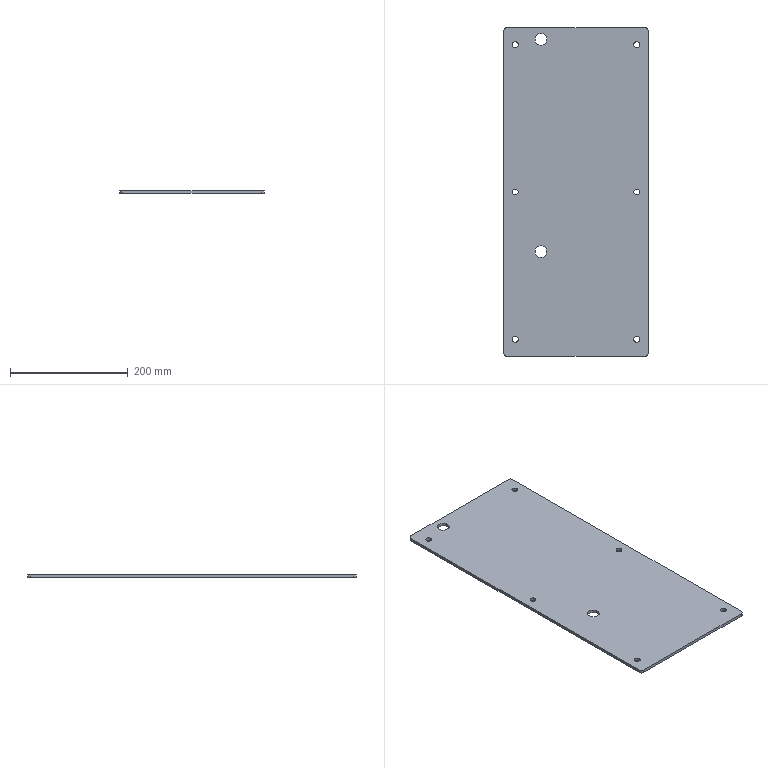Part | SolidWorks | features BaseBody 1 | 1 solid | 26 faces | box 244.5 x 558 x 5 mm | volume 676550 mm3 | cylinder 20 | plane 6 | commonest cylinder face diameters 10 x16 20 x4
STEP:
#1=CARTESIAN_POINT('',(-49.502,-101.,5.));
#2=VERTEX_POINT('',#1);
#3=CARTESIAN_POINT('',(-69.502,-101.,5.));
#4=VERTEX_POINT('',#3);
#5=CARTESIAN_POINT('',(-59.502,-101.,5.));
#6=DIRECTION('',(0.,0.,-1.));
#7=DIRECTION('',(-1.,0.,0.));
#8=AXIS2_PLACEMENT_3D('',#5,#6,#7);
#9=CIRCLE('',#8,10.);
#10=EDGE_CURVE('',#2,#4,#9,.T.);
#11=ORIENTED_EDGE('',*,*,#10,.F.);
#12=CARTESIAN_POINT('',(-49.502,-101.,0.));
#13=VERTEX_POINT('',#12);
#14=CARTESIAN_POINT('',(-49.502,-101.,10.));
#15=DIRECTION('',(0.,0.,-1.));
#16=VECTOR('',#15,1000.);
#17=LINE('',#14,#16);
#18=EDGE_CURVE('',#2,#13,#17,.T.);
#19=ORIENTED_EDGE('',*,*,#18,.T.);
#20=CARTESIAN_POINT('',(-69.502,-101.,0.));
#21=VERTEX_POINT('',#20);
#22=CARTESIAN_POINT('',(-59.502,-101.,0.));
#23=DIRECTION('',(0.,0.,-1.));
#24=DIRECTION('',(-1.,0.,0.));
#25=AXIS2_PLACEMENT_3D('',#22,#23,#24);
#26=CIRCLE('',#25,10.);
#27=EDGE_CURVE('',#13,#21,#26,.T.);
#28=ORIENTED_EDGE('',*,*,#27,.T.);
#29=CARTESIAN_POINT('',(-69.502,-101.,10.));
#30=DIRECTION('',(0.,0.,-1.));
#31=VECTOR('',#30,1000.);
#32=LINE('',#29,#31);
#33=EDGE_CURVE('',#4,#21,#32,.T.);
#34=ORIENTED_EDGE('',*,*,#33,.F.);
#35=EDGE_LOOP('',(#11,#19,#28,#34));
#36=FACE_OUTER_BOUND('',#35,.T.);
#37=CARTESIAN_POINT('',(-59.502,-101.,10.));
#38=DIRECTION('',(0.,0.,-1.));
#39=DIRECTION('',(-1.,0.,0.));
#40=AXIS2_PLACEMENT_3D('',#37,#38,#39);
#41=CYLINDRICAL_SURFACE('',#40,10.);
#42=ADVANCED_FACE('',(#36),#41,.F.);
#43=CARTESIAN_POINT('',(-49.502,259.,5.));
#44=VERTEX_POINT('',#43);
#45=CARTESIAN_POINT('',(-69.502,259.,5.));
#46=VERTEX_POINT('',#45);
#47=CARTESIAN_POINT('',(-59.502,259.,5.));
#48=DIRECTION('',(0.,0.,-1.));
#49=DIRECTION('',(-1.,0.,0.));
#50=AXIS2_PLACEMENT_3D('',#47,#48,#49);
#51=CIRCLE('',#50,10.);
#52=EDGE_CURVE('',#44,#46,#51,.T.);
#53=ORIENTED_EDGE('',*,*,#52,.F.);
#54=CARTESIAN_POINT('',(-49.502,259.,0.));
#55=VERTEX_POINT('',#54);
#56=CARTESIAN_POINT('',(-49.502,259.,10.));
#57=DIRECTION('',(0.,0.,-1.));
#58=VECTOR('',#57,1000.);
#59=LINE('',#56,#58);
#60=EDGE_CURVE('',#44,#55,#59,.T.);
#61=ORIENTED_EDGE('',*,*,#60,.T.);
#62=CARTESIAN_POINT('',(-69.502,259.,0.));
#63=VERTEX_POINT('',#62);
#64=CARTESIAN_POINT('',(-59.502,259.,0.));
#65=DIRECTION('',(0.,0.,-1.));
#66=DIRECTION('',(-1.,0.,0.));
#67=AXIS2_PLACEMENT_3D('',#64,#65,#66);
#68=CIRCLE('',#67,10.);
#69=EDGE_CURVE('',#55,#63,#68,.T.);
#70=ORIENTED_EDGE('',*,*,#69,.T.);
#71=CARTESIAN_POINT('',(-69.502,259.,10.));
#72=DIRECTION('',(0.,0.,-1.));
#73=VECTOR('',#72,1000.);
#74=LINE('',#71,#73);
#75=EDGE_CURVE('',#46,#63,#74,.T.);
#76=ORIENTED_EDGE('',*,*,#75,.F.);
#77=EDGE_LOOP('',(#53,#61,#70,#76));
#78=FACE_OUTER_BOUND('',#77,.T.);
#79=CARTESIAN_POINT('',(-59.502,259.,10.));
#80=DIRECTION('',(0.,0.,-1.));
#81=DIRECTION('',(-1.,0.,0.));
#82=AXIS2_PLACEMENT_3D('',#79,#80,#81);
#83=CYLINDRICAL_SURFACE('',#82,10.);
#84=ADVANCED_FACE('',(#78),#83,.F.);
#85=CARTESIAN_POINT('',(108.25,250.,5.));
#86=VERTEX_POINT('',#85);
#87=CARTESIAN_POINT('',(98.25,250.,5.));
#88=VERTEX_POINT('',#87);
#89=CARTESIAN_POINT('',(103.25,250.,5.));
#90=DIRECTION('',(0.,0.,-1.));
#91=DIRECTION('',(-1.,0.,0.));
#92=AXIS2_PLACEMENT_3D('',#89,#90,#91);
#93=CIRCLE('',#92,5.);
#94=EDGE_CURVE('',#86,#88,#93,.T.);
#95=ORIENTED_EDGE('',*,*,#94,.F.);
#96=CARTESIAN_POINT('',(108.25,250.,0.));
#97=VERTEX_POINT('',#96);
#98=CARTESIAN_POINT('',(108.25,250.,0.));
#99=DIRECTION('',(0.,0.,-1.));
#100=VECTOR('',#99,1000.);
#101=LINE('',#98,#100);
#102=EDGE_CURVE('',#86,#97,#101,.T.);
#103=ORIENTED_EDGE('',*,*,#102,.T.);
#104=CARTESIAN_POINT('',(98.25,250.,0.));
#105=VERTEX_POINT('',#104);
#106=CARTESIAN_POINT('',(103.25,250.,0.));
#107=DIRECTION('',(0.,0.,-1.));
#108=DIRECTION('',(-1.,0.,0.));
#109=AXIS2_PLACEMENT_3D('',#106,#107,#108);
#110=CIRCLE('',#109,5.);
#111=EDGE_CURVE('',#97,#105,#110,.T.);
#112=ORIENTED_EDGE('',*,*,#111,.T.);
#113=CARTESIAN_POINT('',(98.25,250.,0.));
#114=DIRECTION('',(0.,0.,-1.));
#115=VECTOR('',#114,1000.);
#116=LINE('',#113,#115);
#117=EDGE_CURVE('',#88,#105,#116,.T.);
#118=ORIENTED_EDGE('',*,*,#117,.F.);
#119=EDGE_LOOP('',(#95,#103,#112,#118));
#120=FACE_OUTER_BOUND('',#119,.T.);
#121=CARTESIAN_POINT('',(103.25,250.,0.));
#122=DIRECTION('',(0.,0.,-1.));
#123=DIRECTION('',(-1.,0.,0.));
#124=AXIS2_PLACEMENT_3D('',#121,#122,#123);
#125=CYLINDRICAL_SURFACE('',#124,5.);
#126=ADVANCED_FACE('',(#120),#125,.F.);
#127=CARTESIAN_POINT('',(108.25,0.,5.));
#128=VERTEX_POINT('',#127);
#129=CARTESIAN_POINT('',(98.25,0.,5.));
#130=VERTEX_POINT('',#129);
#131=CARTESIAN_POINT('',(103.25,0.,5.));
#132=DIRECTION('',(0.,0.,-1.));
#133=DIRECTION('',(-1.,0.,0.));
#134=AXIS2_PLACEMENT_3D('',#131,#132,#133);
#135=CIRCLE('',#134,5.);
#136=EDGE_CURVE('',#128,#130,#135,.T.);
#137=ORIENTED_EDGE('',*,*,#136,.F.);
#138=CARTESIAN_POINT('',(108.25,0.,0.));
#139=VERTEX_POINT('',#138);
#140=CARTESIAN_POINT('',(108.25,0.,0.));
#141=DIRECTION('',(0.,0.,-1.));
#142=VECTOR('',#141,1000.);
#143=LINE('',#140,#142);
#144=EDGE_CURVE('',#128,#139,#143,.T.);
#145=ORIENTED_EDGE('',*,*,#144,.T.);
#146=CARTESIAN_POINT('',(98.25,0.,0.));
#147=VERTEX_POINT('',#146);
#148=CARTESIAN_POINT('',(103.25,0.,0.));
#149=DIRECTION('',(0.,0.,-1.));
#150=DIRECTION('',(-1.,0.,0.));
#151=AXIS2_PLACEMENT_3D('',#148,#149,#150);
#152=CIRCLE('',#151,5.);
#153=EDGE_CURVE('',#139,#147,#152,.T.);
#154=ORIENTED_EDGE('',*,*,#153,.T.);
#155=CARTESIAN_POINT('',(98.25,0.,0.));
#156=DIRECTION('',(0.,0.,-1.));
#157=VECTOR('',#156,1000.);
#158=LINE('',#155,#157);
#159=EDGE_CURVE('',#130,#147,#158,.T.);
#160=ORIENTED_EDGE('',*,*,#159,.F.);
#161=EDGE_LOOP('',(#137,#145,#154,#160));
#162=FACE_OUTER_BOUND('',#161,.T.);
#163=CARTESIAN_POINT('',(103.25,0.,0.));
#164=DIRECTION('',(0.,0.,-1.));
#165=DIRECTION('',(-1.,0.,0.));
#166=AXIS2_PLACEMENT_3D('',#163,#164,#165);
#167=CYLINDRICAL_SURFACE('',#166,5.);
#168=ADVANCED_FACE('',(#162),#167,.F.);
#169=CARTESIAN_POINT('',(108.25,-250.,5.));
#170=VERTEX_POINT('',#169);
#171=CARTESIAN_POINT('',(98.25,-250.,5.));
#172=VERTEX_POINT('',#171);
#173=CARTESIAN_POINT('',(103.25,-250.,5.));
#174=DIRECTION('',(0.,0.,-1.));
#175=DIRECTION('',(-1.,0.,0.));
#176=AXIS2_PLACEMENT_3D('',#173,#174,#175);
#177=CIRCLE('',#176,5.);
#178=EDGE_CURVE('',#170,#172,#177,.T.);
#179=ORIENTED_EDGE('',*,*,#178,.F.);
#180=CARTESIAN_POINT('',(108.25,-250.,0.));
#181=VERTEX_POINT('',#180);
#182=CARTESIAN_POINT('',(108.25,-250.,0.));
#183=DIRECTION('',(0.,0.,-1.));
#184=VECTOR('',#183,1000.);
#185=LINE('',#182,#184);
#186=EDGE_CURVE('',#170,#181,#185,.T.);
#187=ORIENTED_EDGE('',*,*,#186,.T.);
#188=CARTESIAN_POINT('',(98.25,-250.,0.));
#189=VERTEX_POINT('',#188);
#190=CARTESIAN_POINT('',(103.25,-250.,0.));
#191=DIRECTION('',(0.,0.,-1.));
#192=DIRECTION('',(-1.,0.,0.));
#193=AXIS2_PLACEMENT_3D('',#190,#191,#192);
#194=CIRCLE('',#193,5.);
#195=EDGE_CURVE('',#181,#189,#194,.T.);
#196=ORIENTED_EDGE('',*,*,#195,.T.);
#197=CARTESIAN_POINT('',(98.25,-250.,0.));
#198=DIRECTION('',(0.,0.,-1.));
#199=VECTOR('',#198,1000.);
#200=LINE('',#197,#199);
#201=EDGE_CURVE('',#172,#189,#200,.T.);
#202=ORIENTED_EDGE('',*,*,#201,.F.);
#203=EDGE_LOOP('',(#179,#187,#196,#202));
#204=FACE_OUTER_BOUND('',#203,.T.);
#205=CARTESIAN_POINT('',(103.25,-250.,0.));
#206=DIRECTION('',(0.,0.,-1.));
#207=DIRECTION('',(-1.,0.,0.));
#208=AXIS2_PLACEMENT_3D('',#205,#206,#207);
#209=CYLINDRICAL_SURFACE('',#208,5.);
#210=ADVANCED_FACE('',(#204),#209,.F.);
#211=CARTESIAN_POINT('',(-98.25,-250.,5.));
#212=VERTEX_POINT('',#211);
#213=CARTESIAN_POINT('',(-108.25,-250.,5.));
#214=VERTEX_POINT('',#213);
#215=CARTESIAN_POINT('',(-103.25,-250.,5.));
#216=DIRECTION('',(0.,0.,-1.));
#217=DIRECTION('',(-1.,0.,0.));
#218=AXIS2_PLACEMENT_3D('',#215,#216,#217);
#219=CIRCLE('',#218,5.);
#220=EDGE_CURVE('',#212,#214,#219,.T.);
#221=ORIENTED_EDGE('',*,*,#220,.F.);
#222=CARTESIAN_POINT('',(-98.25,-250.,0.));
#223=VERTEX_POINT('',#222);
#224=CARTESIAN_POINT('',(-98.25,-250.,0.));
#225=DIRECTION('',(0.,0.,-1.));
#226=VECTOR('',#225,1000.);
#227=LINE('',#224,#226);
#228=EDGE_CURVE('',#212,#223,#227,.T.);
#229=ORIENTED_EDGE('',*,*,#228,.T.);
#230=CARTESIAN_POINT('',(-108.25,-250.,0.));
#231=VERTEX_POINT('',#230);
#232=CARTESIAN_POINT('',(-103.25,-250.,0.));
#233=DIRECTION('',(0.,0.,-1.));
#234=DIRECTION('',(-1.,0.,0.));
#235=AXIS2_PLACEMENT_3D('',#232,#233,#234);
#236=CIRCLE('',#235,5.);
#237=EDGE_CURVE('',#223,#231,#236,.T.);
#238=ORIENTED_EDGE('',*,*,#237,.T.);
#239=CARTESIAN_POINT('',(-108.25,-250.,0.));
#240=DIRECTION('',(0.,0.,-1.));
#241=VECTOR('',#240,1000.);
#242=LINE('',#239,#241);
#243=EDGE_CURVE('',#214,#231,#242,.T.);
#244=ORIENTED_EDGE('',*,*,#243,.F.);
#245=EDGE_LOOP('',(#221,#229,#238,#244));
#246=FACE_OUTER_BOUND('',#245,.T.);
#247=CARTESIAN_POINT('',(-103.25,-250.,0.));
#248=DIRECTION('',(0.,0.,-1.));
#249=DIRECTION('',(-1.,0.,0.));
#250=AXIS2_PLACEMENT_3D('',#247,#248,#249);
#251=CYLINDRICAL_SURFACE('',#250,5.);
#252=ADVANCED_FACE('',(#246),#251,.F.);
#253=CARTESIAN_POINT('',(-98.25,0.,5.));
#254=VERTEX_POINT('',#253);
#255=CARTESIAN_POINT('',(-108.25,0.,5.));
#256=VERTEX_POINT('',#255);
#257=CARTESIAN_POINT('',(-103.25,0.,5.));
#258=DIRECTION('',(0.,0.,-1.));
#259=DIRECTION('',(-1.,0.,0.));
#260=AXIS2_PLACEMENT_3D('',#257,#258,#259);
#261=CIRCLE('',#260,5.);
#262=EDGE_CURVE('',#254,#256,#261,.T.);
#263=ORIENTED_EDGE('',*,*,#262,.F.);
#264=CARTESIAN_POINT('',(-98.25,0.,0.));
#265=VERTEX_POINT('',#264);
#266=CARTESIAN_POINT('',(-98.25,0.,0.));
#267=DIRECTION('',(0.,0.,-1.));
#268=VECTOR('',#267,1000.);
#269=LINE('',#266,#268);
#270=EDGE_CURVE('',#254,#265,#269,.T.);
#271=ORIENTED_EDGE('',*,*,#270,.T.);
#272=CARTESIAN_POINT('',(-108.25,0.,0.));
#273=VERTEX_POINT('',#272);
#274=CARTESIAN_POINT('',(-103.25,0.,0.));
#275=DIRECTION('',(0.,0.,-1.));
#276=DIRECTION('',(-1.,0.,0.));
#277=AXIS2_PLACEMENT_3D('',#274,#275,#276);
#278=CIRCLE('',#277,5.);
#279=EDGE_CURVE('',#265,#273,#278,.T.);
#280=ORIENTED_EDGE('',*,*,#279,.T.);
#281=CARTESIAN_POINT('',(-108.25,0.,0.));
#282=DIRECTION('',(0.,0.,-1.));
#283=VECTOR('',#282,1000.);
#284=LINE('',#281,#283);
#285=EDGE_CURVE('',#256,#273,#284,.T.);
#286=ORIENTED_EDGE('',*,*,#285,.F.);
#287=EDGE_LOOP('',(#263,#271,#280,#286));
#288=FACE_OUTER_BOUND('',#287,.T.);
#289=CARTESIAN_POINT('',(-103.25,0.,0.));
#290=DIRECTION('',(0.,0.,-1.));
#291=DIRECTION('',(-1.,0.,0.));
#292=AXIS2_PLACEMENT_3D('',#289,#290,#291);
#293=CYLINDRICAL_SURFACE('',#292,5.);
#294=ADVANCED_FACE('',(#288),#293,.F.);
#295=CARTESIAN_POINT('',(-98.25,250.,5.));
#296=VERTEX_POINT('',#295);
#297=CARTESIAN_POINT('',(-108.25,250.,5.));
#298=VERTEX_POINT('',#297);
#299=CARTESIAN_POINT('',(-103.25,250.,5.));
#300=DIRECTION('',(0.,0.,-1.));
#301=DIRECTION('',(-1.,0.,0.));
#302=AXIS2_PLACEMENT_3D('',#299,#300,#301);
#303=CIRCLE('',#302,5.);
#304=EDGE_CURVE('',#296,#298,#303,.T.);
#305=ORIENTED_EDGE('',*,*,#304,.F.);
#306=CARTESIAN_POINT('',(-98.25,250.,0.));
#307=VERTEX_POINT('',#306);
#308=CARTESIAN_POINT('',(-98.25,250.,0.));
#309=DIRECTION('',(0.,0.,-1.));
#310=VECTOR('',#309,1000.);
#311=LINE('',#308,#310);
#312=EDGE_CURVE('',#296,#307,#311,.T.);
#313=ORIENTED_EDGE('',*,*,#312,.T.);
#314=CARTESIAN_POINT('',(-108.25,250.,0.));
#315=VERTEX_POINT('',#314);
#316=CARTESIAN_POINT('',(-103.25,250.,0.));
#317=DIRECTION('',(0.,0.,-1.));
#318=DIRECTION('',(-1.,0.,0.));
#319=AXIS2_PLACEMENT_3D('',#316,#317,#318);
#320=CIRCLE('',#319,5.);
#321=EDGE_CURVE('',#307,#315,#320,.T.);
#322=ORIENTED_EDGE('',*,*,#321,.T.);
#323=CARTESIAN_POINT('',(-108.25,250.,0.));
#324=DIRECTION('',(0.,0.,-1.));
#325=VECTOR('',#324,1000.);
#326=LINE('',#323,#325);
#327=EDGE_CURVE('',#298,#315,#326,.T.);
#328=ORIENTED_EDGE('',*,*,#327,.F.);
#329=EDGE_LOOP('',(#305,#313,#322,#328));
#330=FACE_OUTER_BOUND('',#329,.T.);
#331=CARTESIAN_POINT('',(-103.25,250.,0.));
#332=DIRECTION('',(0.,0.,-1.));
#333=DIRECTION('',(-1.,0.,0.));
#334=AXIS2_PLACEMENT_3D('',#331,#332,#333);
#335=CYLINDRICAL_SURFACE('',#334,5.);
#336=ADVANCED_FACE('',(#330),#335,.F.);
#337=CARTESIAN_POINT('',(-122.25,274.,0.));
#338=VERTEX_POINT('',#337);
#339=CARTESIAN_POINT('',(-122.25,-274.,0.));
#340=VERTEX_POINT('',#339);
#341=CARTESIAN_POINT('',(-122.25,279.,0.));
#342=DIRECTION('',(0.,-1.,0.));
#343=VECTOR('',#342,1000.);
#344=LINE('',#341,#343);
#345=EDGE_CURVE('',#338,#340,#344,.T.);
#346=ORIENTED_EDGE('',*,*,#345,.T.);
#347=CARTESIAN_POINT('',(-122.25,-274.,5.));
#348=VERTEX_POINT('',#347);
#349=CARTESIAN_POINT('',(-122.25,-274.,5.));
#350=DIRECTION('',(0.,0.,1.));
#351=VECTOR('',#350,1000.);
#352=LINE('',#349,#351);
#353=EDGE_CURVE('',#340,#348,#352,.T.);
#354=ORIENTED_EDGE('',*,*,#353,.T.);
#355=CARTESIAN_POINT('',(-122.25,274.,5.));
#356=VERTEX_POINT('',#355);
#357=CARTESIAN_POINT('',(-122.25,279.,5.));
#358=DIRECTION('',(0.,-1.,0.));
#359=VECTOR('',#358,1000.);
#360=LINE('',#357,#359);
#361=EDGE_CURVE('',#356,#348,#360,.T.);
#362=ORIENTED_EDGE('',*,*,#361,.F.);
#363=CARTESIAN_POINT('',(-122.25,274.,5.));
#364=DIRECTION('',(0.,0.,-1.));
#365=VECTOR('',#364,1000.);
#366=LINE('',#363,#365);
#367=EDGE_CURVE('',#356,#338,#366,.T.);
#368=ORIENTED_EDGE('',*,*,#367,.T.);
#369=EDGE_LOOP('',(#346,#354,#362,#368));
#370=FACE_OUTER_BOUND('',#369,.T.);
#371=CARTESIAN_POINT('',(-122.25,279.,5.));
#372=DIRECTION('',(1.,0.,0.));
#373=DIRECTION('',(0.,1.,0.));
#374=AXIS2_PLACEMENT_3D('',#371,#372,#373);
#375=PLANE('',#374);
#376=ADVANCED_FACE('',(#370),#375,.F.);
#377=CARTESIAN_POINT('',(-117.25,-279.,0.));
#378=VERTEX_POINT('',#377);
#379=CARTESIAN_POINT('',(117.25,-279.,0.));
#380=VERTEX_POINT('',#379);
#381=CARTESIAN_POINT('',(122.25,-279.,0.));
#382=DIRECTION('',(1.,0.,0.));
#383=VECTOR('',#382,1000.);
#384=LINE('',#381,#383);
#385=EDGE_CURVE('',#378,#380,#384,.T.);
#386=ORIENTED_EDGE('',*,*,#385,.T.);
#387=CARTESIAN_POINT('',(117.25,-279.,5.));
#388=VERTEX_POINT('',#387);
#389=CARTESIAN_POINT('',(117.25,-279.,5.));
#390=DIRECTION('',(0.,0.,1.));
#391=VECTOR('',#390,1000.);
#392=LINE('',#389,#391);
#393=EDGE_CURVE('',#380,#388,#392,.T.);
#394=ORIENTED_EDGE('',*,*,#393,.T.);
#395=CARTESIAN_POINT('',(-117.25,-279.,5.));
#396=VERTEX_POINT('',#395);
#397=CARTESIAN_POINT('',(122.25,-279.,5.));
#398=DIRECTION('',(1.,0.,0.));
#399=VECTOR('',#398,1000.);
#400=LINE('',#397,#399);
#401=EDGE_CURVE('',#396,#388,#400,.T.);
#402=ORIENTED_EDGE('',*,*,#401,.F.);
#403=CARTESIAN_POINT('',(-117.25,-279.,5.));
#404=DIRECTION('',(0.,0.,-1.));
#405=VECTOR('',#404,1000.);
#406=LINE('',#403,#405);
#407=EDGE_CURVE('',#396,#378,#406,.T.);
#408=ORIENTED_EDGE('',*,*,#407,.T.);
#409=EDGE_LOOP('',(#386,#394,#402,#408));
#410=FACE_OUTER_BOUND('',#409,.T.);
#411=CARTESIAN_POINT('',(122.25,-279.,5.));
#412=DIRECTION('',(0.,1.,0.));
#413=DIRECTION('',(0.,0.,1.));
#414=AXIS2_PLACEMENT_3D('',#411,#412,#413);
#415=PLANE('',#414);
#416=ADVANCED_FACE('',(#410),#415,.F.);
#417=CARTESIAN_POINT('',(122.25,-274.,5.));
#418=VERTEX_POINT('',#417);
#419=CARTESIAN_POINT('',(122.25,274.,5.));
#420=VERTEX_POINT('',#419);
#421=CARTESIAN_POINT('',(122.25,279.,5.));
#422=DIRECTION('',(0.,1.,0.));
#423=VECTOR('',#422,1000.);
#424=LINE('',#421,#423);
#425=EDGE_CURVE('',#418,#420,#424,.T.);
#426=ORIENTED_EDGE('',*,*,#425,.F.);
#427=CARTESIAN_POINT('',(122.25,-274.,0.));
#428=VERTEX_POINT('',#427);
#429=CARTESIAN_POINT('',(122.25,-274.,5.));
#430=DIRECTION('',(0.,0.,-1.));
#431=VECTOR('',#430,1000.);
#432=LINE('',#429,#431);
#433=EDGE_CURVE('',#418,#428,#432,.T.);
#434=ORIENTED_EDGE('',*,*,#433,.T.);
#435=CARTESIAN_POINT('',(122.25,274.,0.));
#436=VERTEX_POINT('',#435);
#437=CARTESIAN_POINT('',(122.25,279.,0.));
#438=DIRECTION('',(0.,1.,0.));
#439=VECTOR('',#438,1000.);
#440=LINE('',#437,#439);
#441=EDGE_CURVE('',#428,#436,#440,.T.);
#442=ORIENTED_EDGE('',*,*,#441,.T.);
#443=CARTESIAN_POINT('',(122.25,274.,5.));
#444=DIRECTION('',(0.,0.,1.));
#445=VECTOR('',#444,1000.);
#446=LINE('',#443,#445);
#447=EDGE_CURVE('',#436,#420,#446,.T.);
#448=ORIENTED_EDGE('',*,*,#447,.T.);
#449=EDGE_LOOP('',(#426,#434,#442,#448));
#450=FACE_OUTER_BOUND('',#449,.T.);
#451=CARTESIAN_POINT('',(122.25,279.,5.));
#452=DIRECTION('',(-1.,0.,0.));
#453=DIRECTION('',(0.,-1.,0.));
#454=AXIS2_PLACEMENT_3D('',#451,#452,#453);
#455=PLANE('',#454);
#456=ADVANCED_FACE('',(#450),#455,.F.);
#457=CARTESIAN_POINT('',(117.25,279.,5.));
#458=VERTEX_POINT('',#457);
#459=CARTESIAN_POINT('',(-117.25,279.,5.));
#460=VERTEX_POINT('',#459);
#461=CARTESIAN_POINT('',(122.25,279.,5.));
#462=DIRECTION('',(-1.,0.,0.));
#463=VECTOR('',#462,1000.);
#464=LINE('',#461,#463);
#465=EDGE_CURVE('',#458,#460,#464,.T.);
#466=ORIENTED_EDGE('',*,*,#465,.F.);
#467=CARTESIAN_POINT('',(117.25,279.,0.));
#468=VERTEX_POINT('',#467);
#469=CARTESIAN_POINT('',(117.25,279.,5.));
#470=DIRECTION('',(0.,0.,-1.));
#471=VECTOR('',#470,1000.);
#472=LINE('',#469,#471);
#473=EDGE_CURVE('',#458,#468,#472,.T.);
#474=ORIENTED_EDGE('',*,*,#473,.T.);
#475=CARTESIAN_POINT('',(-117.25,279.,0.));
#476=VERTEX_POINT('',#475);
#477=CARTESIAN_POINT('',(122.25,279.,0.));
#478=DIRECTION('',(-1.,0.,0.));
#479=VECTOR('',#478,1000.);
#480=LINE('',#477,#479);
#481=EDGE_CURVE('',#468,#476,#480,.T.);
#482=ORIENTED_EDGE('',*,*,#481,.T.);
#483=CARTESIAN_POINT('',(-117.25,279.,5.));
#484=DIRECTION('',(0.,0.,1.));
#485=VECTOR('',#484,1000.);
#486=LINE('',#483,#485);
#487=EDGE_CURVE('',#476,#460,#486,.T.);
#488=ORIENTED_EDGE('',*,*,#487,.T.);
#489=EDGE_LOOP('',(#466,#474,#482,#488));
#490=FACE_OUTER_BOUND('',#489,.T.);
#491=CARTESIAN_POINT('',(122.25,279.,5.));
#492=DIRECTION('',(0.,-1.,0.));
#493=DIRECTION('',(1.,0.,0.));
#494=AXIS2_PLACEMENT_3D('',#491,#492,#493);
#495=PLANE('',#494);
#496=ADVANCED_FACE('',(#490),#495,.F.);
#497=CARTESIAN_POINT('',(-59.502,-101.,5.));
#498=DIRECTION('',(0.,0.,-1.));
#499=DIRECTION('',(-1.,0.,0.));
#500=AXIS2_PLACEMENT_3D('',#497,#498,#499);
#501=CIRCLE('',#500,10.);
#502=EDGE_CURVE('',#4,#2,#501,.T.);
#503=ORIENTED_EDGE('',*,*,#502,.T.);
#504=ORIENTED_EDGE('',*,*,#10,.T.);
#505=EDGE_LOOP('',(#503,#504));
#506=FACE_BOUND('',#505,.T.);
#507=CARTESIAN_POINT('',(-59.502,259.,5.));
#508=DIRECTION('',(0.,0.,-1.));
#509=DIRECTION('',(-1.,0.,0.));
#510=AXIS2_PLACEMENT_3D('',#507,#508,#509);
#511=CIRCLE('',#510,10.);
#512=EDGE_CURVE('',#46,#44,#511,.T.);
#513=ORIENTED_EDGE('',*,*,#512,.T.);
#514=ORIENTED_EDGE('',*,*,#52,.T.);
#515=EDGE_LOOP('',(#513,#514));
#516=FACE_BOUND('',#515,.T.);
#517=CARTESIAN_POINT('',(103.25,250.,5.));
#518=DIRECTION('',(0.,0.,-1.));
#519=DIRECTION('',(-1.,0.,0.));
#520=AXIS2_PLACEMENT_3D('',#517,#518,#519);
#521=CIRCLE('',#520,5.);
#522=EDGE_CURVE('',#88,#86,#521,.T.);
#523=ORIENTED_EDGE('',*,*,#522,.T.);
#524=ORIENTED_EDGE('',*,*,#94,.T.);
#525=EDGE_LOOP('',(#523,#524));
#526=FACE_BOUND('',#525,.T.);
#527=CARTESIAN_POINT('',(103.25,0.,5.));
#528=DIRECTION('',(0.,0.,-1.));
#529=DIRECTION('',(-1.,0.,0.));
#530=AXIS2_PLACEMENT_3D('',#527,#528,#529);
#531=CIRCLE('',#530,5.);
#532=EDGE_CURVE('',#130,#128,#531,.T.);
#533=ORIENTED_EDGE('',*,*,#532,.T.);
#534=ORIENTED_EDGE('',*,*,#136,.T.);
#535=EDGE_LOOP('',(#533,#534));
#536=FACE_BOUND('',#535,.T.);
#537=CARTESIAN_POINT('',(103.25,-250.,5.));
#538=DIRECTION('',(0.,0.,-1.));
#539=DIRECTION('',(-1.,0.,0.));
#540=AXIS2_PLACEMENT_3D('',#537,#538,#539);
#541=CIRCLE('',#540,5.);
#542=EDGE_CURVE('',#172,#170,#541,.T.);
#543=ORIENTED_EDGE('',*,*,#542,.T.);
#544=ORIENTED_EDGE('',*,*,#178,.T.);
#545=EDGE_LOOP('',(#543,#544));
#546=FACE_BOUND('',#545,.T.);
#547=CARTESIAN_POINT('',(-103.25,-250.,5.));
#548=DIRECTION('',(0.,0.,-1.));
#549=DIRECTION('',(-1.,0.,0.));
#550=AXIS2_PLACEMENT_3D('',#547,#548,#549);
#551=CIRCLE('',#550,5.);
#552=EDGE_CURVE('',#214,#212,#551,.T.);
#553=ORIENTED_EDGE('',*,*,#552,.T.);
#554=ORIENTED_EDGE('',*,*,#220,.T.);
#555=EDGE_LOOP('',(#553,#554));
#556=FACE_BOUND('',#555,.T.);
#557=CARTESIAN_POINT('',(-103.25,0.,5.));
#558=DIRECTION('',(0.,0.,-1.));
#559=DIRECTION('',(-1.,0.,0.));
#560=AXIS2_PLACEMENT_3D('',#557,#558,#559);
#561=CIRCLE('',#560,5.);
#562=EDGE_CURVE('',#256,#254,#561,.T.);
#563=ORIENTED_EDGE('',*,*,#562,.T.);
#564=ORIENTED_EDGE('',*,*,#262,.T.);
#565=EDGE_LOOP('',(#563,#564));
#566=FACE_BOUND('',#565,.T.);
#567=CARTESIAN_POINT('',(-103.25,250.,5.));
#568=DIRECTION('',(0.,0.,-1.));
#569=DIRECTION('',(-1.,0.,0.));
#570=AXIS2_PLACEMENT_3D('',#567,#568,#569);
#571=CIRCLE('',#570,5.);
#572=EDGE_CURVE('',#298,#296,#571,.T.);
#573=ORIENTED_EDGE('',*,*,#572,.T.);
#574=ORIENTED_EDGE('',*,*,#304,.T.);
#575=EDGE_LOOP('',(#573,#574));
#576=FACE_BOUND('',#575,.T.);
#577=ORIENTED_EDGE('',*,*,#401,.T.);
#578=CARTESIAN_POINT('',(117.25,-274.,5.));
#579=DIRECTION('',(0.,0.,1.));
#580=DIRECTION('',(-1.,0.,0.));
#581=AXIS2_PLACEMENT_3D('',#578,#579,#580);
#582=CIRCLE('',#581,5.);
#583=EDGE_CURVE('',#388,#418,#582,.T.);
#584=ORIENTED_EDGE('',*,*,#583,.T.);
#585=ORIENTED_EDGE('',*,*,#425,.T.);
#586=CARTESIAN_POINT('',(117.25,274.,5.));
#587=DIRECTION('',(0.,0.,1.));
#588=DIRECTION('',(-1.,0.,0.));
#589=AXIS2_PLACEMENT_3D('',#586,#587,#588);
#590=CIRCLE('',#589,5.);
#591=EDGE_CURVE('',#420,#458,#590,.T.);
#592=ORIENTED_EDGE('',*,*,#591,.T.);
#593=ORIENTED_EDGE('',*,*,#465,.T.);
#594=CARTESIAN_POINT('',(-117.25,274.,5.));
#595=DIRECTION('',(0.,0.,1.));
#596=DIRECTION('',(-1.,0.,0.));
#597=AXIS2_PLACEMENT_3D('',#594,#595,#596);
#598=CIRCLE('',#597,5.);
#599=EDGE_CURVE('',#460,#356,#598,.T.);
#600=ORIENTED_EDGE('',*,*,#599,.T.);
#601=ORIENTED_EDGE('',*,*,#361,.T.);
#602=CARTESIAN_POINT('',(-117.25,-274.,5.));
#603=DIRECTION('',(0.,0.,1.));
#604=DIRECTION('',(-1.,0.,0.));
#605=AXIS2_PLACEMENT_3D('',#602,#603,#604);
#606=CIRCLE('',#605,5.);
#607=EDGE_CURVE('',#348,#396,#606,.T.);
#608=ORIENTED_EDGE('',*,*,#607,.T.);
#609=EDGE_LOOP('',(#577,#584,#585,#592,#593,#600,#601,#608));
#610=FACE_OUTER_BOUND('',#609,.T.);
#611=CARTESIAN_POINT('',(0.,0.,5.));
#612=DIRECTION('',(0.,0.,-1.));
#613=DIRECTION('',(-1.,0.,0.));
#614=AXIS2_PLACEMENT_3D('',#611,#612,#613);
#615=PLANE('',#614);
#616=ADVANCED_FACE('',(#506,#516,#526,#536,#546,#556,#566,#576,#610),#615,.F.);
#617=CARTESIAN_POINT('',(-59.502,-101.,0.));
#618=DIRECTION('',(0.,0.,-1.));
#619=DIRECTION('',(-1.,0.,0.));
#620=AXIS2_PLACEMENT_3D('',#617,#618,#619);
#621=CIRCLE('',#620,10.);
#622=EDGE_CURVE('',#21,#13,#621,.T.);
#623=ORIENTED_EDGE('',*,*,#622,.F.);
#624=ORIENTED_EDGE('',*,*,#27,.F.);
#625=EDGE_LOOP('',(#623,#624));
#626=FACE_BOUND('',#625,.T.);
#627=CARTESIAN_POINT('',(-59.502,259.,0.));
#628=DIRECTION('',(0.,0.,-1.));
#629=DIRECTION('',(-1.,0.,0.));
#630=AXIS2_PLACEMENT_3D('',#627,#628,#629);
#631=CIRCLE('',#630,10.);
#632=EDGE_CURVE('',#63,#55,#631,.T.);
#633=ORIENTED_EDGE('',*,*,#632,.F.);
#634=ORIENTED_EDGE('',*,*,#69,.F.);
#635=EDGE_LOOP('',(#633,#634));
#636=FACE_BOUND('',#635,.T.);
#637=CARTESIAN_POINT('',(103.25,250.,0.));
#638=DIRECTION('',(0.,0.,-1.));
#639=DIRECTION('',(-1.,0.,0.));
#640=AXIS2_PLACEMENT_3D('',#637,#638,#639);
#641=CIRCLE('',#640,5.);
#642=EDGE_CURVE('',#105,#97,#641,.T.);
#643=ORIENTED_EDGE('',*,*,#642,.F.);
#644=ORIENTED_EDGE('',*,*,#111,.F.);
#645=EDGE_LOOP('',(#643,#644));
#646=FACE_BOUND('',#645,.T.);
#647=CARTESIAN_POINT('',(103.25,0.,0.));
#648=DIRECTION('',(0.,0.,-1.));
#649=DIRECTION('',(-1.,0.,0.));
#650=AXIS2_PLACEMENT_3D('',#647,#648,#649);
#651=CIRCLE('',#650,5.);
#652=EDGE_CURVE('',#147,#139,#651,.T.);
#653=ORIENTED_EDGE('',*,*,#652,.F.);
#654=ORIENTED_EDGE('',*,*,#153,.F.);
#655=EDGE_LOOP('',(#653,#654));
#656=FACE_BOUND('',#655,.T.);
#657=CARTESIAN_POINT('',(103.25,-250.,0.));
#658=DIRECTION('',(0.,0.,-1.));
#659=DIRECTION('',(-1.,0.,0.));
#660=AXIS2_PLACEMENT_3D('',#657,#658,#659);
#661=CIRCLE('',#660,5.);
#662=EDGE_CURVE('',#189,#181,#661,.T.);
#663=ORIENTED_EDGE('',*,*,#662,.F.);
#664=ORIENTED_EDGE('',*,*,#195,.F.);
#665=EDGE_LOOP('',(#663,#664));
#666=FACE_BOUND('',#665,.T.);
#667=CARTESIAN_POINT('',(-103.25,-250.,0.));
#668=DIRECTION('',(0.,0.,-1.));
#669=DIRECTION('',(-1.,0.,0.));
#670=AXIS2_PLACEMENT_3D('',#667,#668,#669);
#671=CIRCLE('',#670,5.);
#672=EDGE_CURVE('',#231,#223,#671,.T.);
#673=ORIENTED_EDGE('',*,*,#672,.F.);
#674=ORIENTED_EDGE('',*,*,#237,.F.);
#675=EDGE_LOOP('',(#673,#674));
#676=FACE_BOUND('',#675,.T.);
#677=CARTESIAN_POINT('',(-103.25,0.,0.));
#678=DIRECTION('',(0.,0.,-1.));
#679=DIRECTION('',(-1.,0.,0.));
#680=AXIS2_PLACEMENT_3D('',#677,#678,#679);
#681=CIRCLE('',#680,5.);
#682=EDGE_CURVE('',#273,#265,#681,.T.);
#683=ORIENTED_EDGE('',*,*,#682,.F.);
#684=ORIENTED_EDGE('',*,*,#279,.F.);
#685=EDGE_LOOP('',(#683,#684));
#686=FACE_BOUND('',#685,.T.);
#687=CARTESIAN_POINT('',(-103.25,250.,0.));
#688=DIRECTION('',(0.,0.,-1.));
#689=DIRECTION('',(-1.,0.,0.));
#690=AXIS2_PLACEMENT_3D('',#687,#688,#689);
#691=CIRCLE('',#690,5.);
#692=EDGE_CURVE('',#315,#307,#691,.T.);
#693=ORIENTED_EDGE('',*,*,#692,.F.);
#694=ORIENTED_EDGE('',*,*,#321,.F.);
#695=EDGE_LOOP('',(#693,#694));
#696=FACE_BOUND('',#695,.T.);
#697=ORIENTED_EDGE('',*,*,#441,.F.);
#698=CARTESIAN_POINT('',(117.25,-274.,0.));
#699=DIRECTION('',(0.,0.,-1.));
#700=DIRECTION('',(-1.,0.,0.));
#701=AXIS2_PLACEMENT_3D('',#698,#699,#700);
#702=CIRCLE('',#701,5.);
#703=EDGE_CURVE('',#428,#380,#702,.T.);
#704=ORIENTED_EDGE('',*,*,#703,.T.);
#705=ORIENTED_EDGE('',*,*,#385,.F.);
#706=CARTESIAN_POINT('',(-117.25,-274.,0.));
#707=DIRECTION('',(0.,0.,-1.));
#708=DIRECTION('',(-1.,0.,0.));
#709=AXIS2_PLACEMENT_3D('',#706,#707,#708);
#710=CIRCLE('',#709,5.);
#711=EDGE_CURVE('',#378,#340,#710,.T.);
#712=ORIENTED_EDGE('',*,*,#711,.T.);
#713=ORIENTED_EDGE('',*,*,#345,.F.);
#714=CARTESIAN_POINT('',(-117.25,274.,0.));
#715=DIRECTION('',(0.,0.,-1.));
#716=DIRECTION('',(-1.,0.,0.));
#717=AXIS2_PLACEMENT_3D('',#714,#715,#716);
#718=CIRCLE('',#717,5.);
#719=EDGE_CURVE('',#338,#476,#718,.T.);
#720=ORIENTED_EDGE('',*,*,#719,.T.);
#721=ORIENTED_EDGE('',*,*,#481,.F.);
#722=CARTESIAN_POINT('',(117.25,274.,0.));
#723=DIRECTION('',(0.,0.,-1.));
#724=DIRECTION('',(-1.,0.,0.));
#725=AXIS2_PLACEMENT_3D('',#722,#723,#724);
#726=CIRCLE('',#725,5.);
#727=EDGE_CURVE('',#468,#436,#726,.T.);
#728=ORIENTED_EDGE('',*,*,#727,.T.);
#729=EDGE_LOOP('',(#697,#704,#705,#712,#713,#720,#721,#728));
#730=FACE_OUTER_BOUND('',#729,.T.);
#731=CARTESIAN_POINT('',(0.,0.,0.));
#732=DIRECTION('',(0.,0.,-1.));
#733=DIRECTION('',(-1.,0.,0.));
#734=AXIS2_PLACEMENT_3D('',#731,#732,#733);
#735=PLANE('',#734);
#736=ADVANCED_FACE('',(#626,#636,#646,#656,#666,#676,#686,#696,#730),#735,.T.);
#737=ORIENTED_EDGE('',*,*,#583,.F.);
#738=ORIENTED_EDGE('',*,*,#393,.F.);
#739=ORIENTED_EDGE('',*,*,#703,.F.);
#740=ORIENTED_EDGE('',*,*,#433,.F.);
#741=EDGE_LOOP('',(#737,#738,#739,#740));
#742=FACE_OUTER_BOUND('',#741,.T.);
#743=CARTESIAN_POINT('',(117.25,-274.,5.));
#744=DIRECTION('',(0.,0.,-1.));
#745=DIRECTION('',(-1.,0.,0.));
#746=AXIS2_PLACEMENT_3D('',#743,#744,#745);
#747=CYLINDRICAL_SURFACE('',#746,5.);
#748=ADVANCED_FACE('',(#742),#747,.T.);
#749=ORIENTED_EDGE('',*,*,#607,.F.);
#750=ORIENTED_EDGE('',*,*,#353,.F.);
#751=ORIENTED_EDGE('',*,*,#711,.F.);
#752=ORIENTED_EDGE('',*,*,#407,.F.);
#753=EDGE_LOOP('',(#749,#750,#751,#752));
#754=FACE_OUTER_BOUND('',#753,.T.);
#755=CARTESIAN_POINT('',(-117.25,-274.,5.));
#756=DIRECTION('',(0.,0.,-1.));
#757=DIRECTION('',(-1.,0.,0.));
#758=AXIS2_PLACEMENT_3D('',#755,#756,#757);
#759=CYLINDRICAL_SURFACE('',#758,5.);
#760=ADVANCED_FACE('',(#754),#759,.T.);
#761=ORIENTED_EDGE('',*,*,#591,.F.);
#762=ORIENTED_EDGE('',*,*,#447,.F.);
#763=ORIENTED_EDGE('',*,*,#727,.F.);
#764=ORIENTED_EDGE('',*,*,#473,.F.);
#765=EDGE_LOOP('',(#761,#762,#763,#764));
#766=FACE_OUTER_BOUND('',#765,.T.);
#767=CARTESIAN_POINT('',(117.25,274.,5.));
#768=DIRECTION('',(0.,0.,-1.));
#769=DIRECTION('',(-1.,0.,0.));
#770=AXIS2_PLACEMENT_3D('',#767,#768,#769);
#771=CYLINDRICAL_SURFACE('',#770,5.);
#772=ADVANCED_FACE('',(#766),#771,.T.);
#773=ORIENTED_EDGE('',*,*,#599,.F.);
#774=ORIENTED_EDGE('',*,*,#487,.F.);
#775=ORIENTED_EDGE('',*,*,#719,.F.);
#776=ORIENTED_EDGE('',*,*,#367,.F.);
#777=EDGE_LOOP('',(#773,#774,#775,#776));
#778=FACE_OUTER_BOUND('',#777,.T.);
#779=CARTESIAN_POINT('',(-117.25,274.,5.));
#780=DIRECTION('',(0.,0.,-1.));
#781=DIRECTION('',(-1.,0.,0.));
#782=AXIS2_PLACEMENT_3D('',#779,#780,#781);
#783=CYLINDRICAL_SURFACE('',#782,5.);
#784=ADVANCED_FACE('',(#778),#783,.T.);
#785=ORIENTED_EDGE('',*,*,#312,.F.);
#786=ORIENTED_EDGE('',*,*,#572,.F.);
#787=ORIENTED_EDGE('',*,*,#327,.T.);
#788=ORIENTED_EDGE('',*,*,#692,.T.);
#789=EDGE_LOOP('',(#785,#786,#787,#788));
#790=FACE_OUTER_BOUND('',#789,.T.);
#791=CARTESIAN_POINT('',(-103.25,250.,0.));
#792=DIRECTION('',(0.,0.,-1.));
#793=DIRECTION('',(-1.,0.,0.));
#794=AXIS2_PLACEMENT_3D('',#791,#792,#793);
#795=CYLINDRICAL_SURFACE('',#794,5.);
#796=ADVANCED_FACE('',(#790),#795,.F.);
#797=ORIENTED_EDGE('',*,*,#270,.F.);
#798=ORIENTED_EDGE('',*,*,#562,.F.);
#799=ORIENTED_EDGE('',*,*,#285,.T.);
#800=ORIENTED_EDGE('',*,*,#682,.T.);
#801=EDGE_LOOP('',(#797,#798,#799,#800));
#802=FACE_OUTER_BOUND('',#801,.T.);
#803=CARTESIAN_POINT('',(-103.25,0.,0.));
#804=DIRECTION('',(0.,0.,-1.));
#805=DIRECTION('',(-1.,0.,0.));
#806=AXIS2_PLACEMENT_3D('',#803,#804,#805);
#807=CYLINDRICAL_SURFACE('',#806,5.);
#808=ADVANCED_FACE('',(#802),#807,.F.);
#809=ORIENTED_EDGE('',*,*,#228,.F.);
#810=ORIENTED_EDGE('',*,*,#552,.F.);
#811=ORIENTED_EDGE('',*,*,#243,.T.);
#812=ORIENTED_EDGE('',*,*,#672,.T.);
#813=EDGE_LOOP('',(#809,#810,#811,#812));
#814=FACE_OUTER_BOUND('',#813,.T.);
#815=CARTESIAN_POINT('',(-103.25,-250.,0.));
#816=DIRECTION('',(0.,0.,-1.));
#817=DIRECTION('',(-1.,0.,0.));
#818=AXIS2_PLACEMENT_3D('',#815,#816,#817);
#819=CYLINDRICAL_SURFACE('',#818,5.);
#820=ADVANCED_FACE('',(#814),#819,.F.);
#821=ORIENTED_EDGE('',*,*,#186,.F.);
#822=ORIENTED_EDGE('',*,*,#542,.F.);
#823=ORIENTED_EDGE('',*,*,#201,.T.);
#824=ORIENTED_EDGE('',*,*,#662,.T.);
#825=EDGE_LOOP('',(#821,#822,#823,#824));
#826=FACE_OUTER_BOUND('',#825,.T.);
#827=CARTESIAN_POINT('',(103.25,-250.,0.));
#828=DIRECTION('',(0.,0.,-1.));
#829=DIRECTION('',(-1.,0.,0.));
#830=AXIS2_PLACEMENT_3D('',#827,#828,#829);
#831=CYLINDRICAL_SURFACE('',#830,5.);
#832=ADVANCED_FACE('',(#826),#831,.F.);
#833=ORIENTED_EDGE('',*,*,#144,.F.);
#834=ORIENTED_EDGE('',*,*,#532,.F.);
#835=ORIENTED_EDGE('',*,*,#159,.T.);
#836=ORIENTED_EDGE('',*,*,#652,.T.);
#837=EDGE_LOOP('',(#833,#834,#835,#836));
#838=FACE_OUTER_BOUND('',#837,.T.);
#839=CARTESIAN_POINT('',(103.25,0.,0.));
#840=DIRECTION('',(0.,0.,-1.));
#841=DIRECTION('',(-1.,0.,0.));
#842=AXIS2_PLACEMENT_3D('',#839,#840,#841);
#843=CYLINDRICAL_SURFACE('',#842,5.);
#844=ADVANCED_FACE('',(#838),#843,.F.);
#845=ORIENTED_EDGE('',*,*,#102,.F.);
#846=ORIENTED_EDGE('',*,*,#522,.F.);
#847=ORIENTED_EDGE('',*,*,#117,.T.);
#848=ORIENTED_EDGE('',*,*,#642,.T.);
#849=EDGE_LOOP('',(#845,#846,#847,#848));
#850=FACE_OUTER_BOUND('',#849,.T.);
#851=CARTESIAN_POINT('',(103.25,250.,0.));
#852=DIRECTION('',(0.,0.,-1.));
#853=DIRECTION('',(-1.,0.,0.));
#854=AXIS2_PLACEMENT_3D('',#851,#852,#853);
#855=CYLINDRICAL_SURFACE('',#854,5.);
#856=ADVANCED_FACE('',(#850),#855,.F.);
#857=ORIENTED_EDGE('',*,*,#60,.F.);
#858=ORIENTED_EDGE('',*,*,#512,.F.);
#859=ORIENTED_EDGE('',*,*,#75,.T.);
#860=ORIENTED_EDGE('',*,*,#632,.T.);
#861=EDGE_LOOP('',(#857,#858,#859,#860));
#862=FACE_OUTER_BOUND('',#861,.T.);
#863=CARTESIAN_POINT('',(-59.502,259.,10.));
#864=DIRECTION('',(0.,0.,-1.));
#865=DIRECTION('',(-1.,0.,0.));
#866=AXIS2_PLACEMENT_3D('',#863,#864,#865);
#867=CYLINDRICAL_SURFACE('',#866,10.);
#868=ADVANCED_FACE('',(#862),#867,.F.);
#869=ORIENTED_EDGE('',*,*,#18,.F.);
#870=ORIENTED_EDGE('',*,*,#502,.F.);
#871=ORIENTED_EDGE('',*,*,#33,.T.);
#872=ORIENTED_EDGE('',*,*,#622,.T.);
#873=EDGE_LOOP('',(#869,#870,#871,#872));
#874=FACE_OUTER_BOUND('',#873,.T.);
#875=CARTESIAN_POINT('',(-59.502,-101.,10.));
#876=DIRECTION('',(0.,0.,-1.));
#877=DIRECTION('',(-1.,0.,0.));
#878=AXIS2_PLACEMENT_3D('',#875,#876,#877);
#879=CYLINDRICAL_SURFACE('',#878,10.);
#880=ADVANCED_FACE('',(#874),#879,.F.);
#881=CLOSED_SHELL('',(#42,#84,#126,#168,#210,#252,#294,#336,#376,#416,#456,#496,#616,#736,#748,#760,#772,#784,#796,#808,#820,#832,#844,#856,#868,#880));
#882=MANIFOLD_SOLID_BREP('',#881);
#883=CARTESIAN_POINT('',(0.,0.,0.));
#884=DIRECTION('',(0.,0.,1.));
#885=DIRECTION('',(1.,0.,0.));
#886=AXIS2_PLACEMENT_3D('',#883,#884,#885);
#887=(LENGTH_UNIT()NAMED_UNIT(*)SI_UNIT(.MILLI.,.METRE.));
#888=UNCERTAINTY_MEASURE_WITH_UNIT(LENGTH_MEASURE(0.00001),#887,'','');
#889=(NAMED_UNIT(*)PLANE_ANGLE_UNIT()SI_UNIT($,.RADIAN.));
#890=(NAMED_UNIT(*)SI_UNIT($,.STERADIAN.)SOLID_ANGLE_UNIT());
#891=(GEOMETRIC_REPRESENTATION_CONTEXT(3)GLOBAL_UNCERTAINTY_ASSIGNED_CONTEXT((#888))GLOBAL_UNIT_ASSIGNED_CONTEXT((#887,#889,#890))REPRESENTATION_CONTEXT('',''));
#892=ADVANCED_BREP_SHAPE_REPRESENTATION('',(#882,#886),#891);